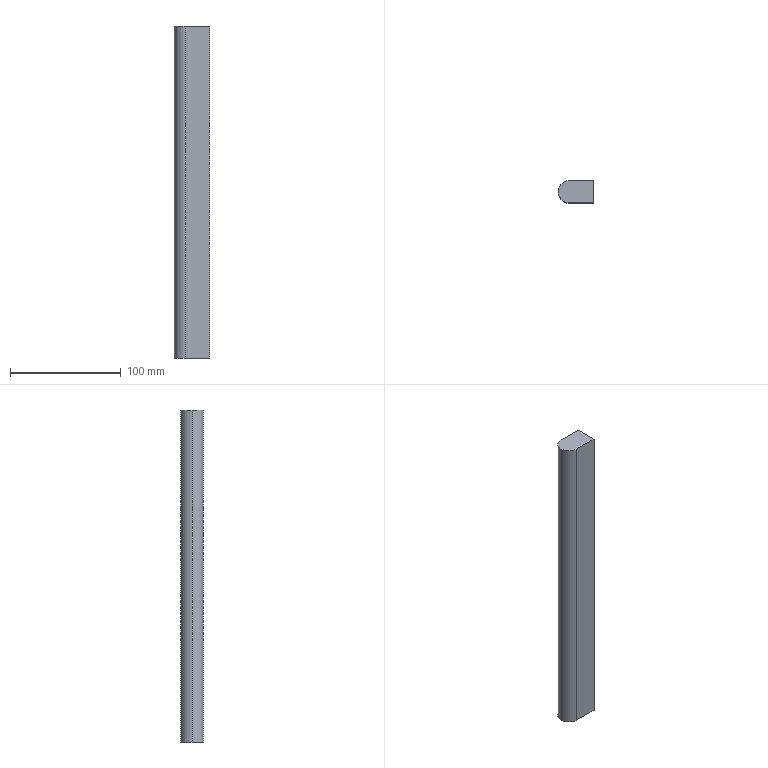Part | STEP file | Part 9 | 1 solid | 7 faces | box 32 x 20 x 300 mm | volume 179124 mm3 | plane 5 | cylinder 2 | commonest cylinder face diameters 20 x2
STEP:
#1=CARTESIAN_POINT('',(-10.,0.,300.));
#2=VERTEX_POINT('',#1);
#3=CARTESIAN_POINT('',(0.,-10.,300.));
#4=VERTEX_POINT('',#3);
#5=CARTESIAN_POINT('',(0.,0.,300.));
#6=DIRECTION('',(0.,0.,1.));
#7=DIRECTION('',(1.,0.,0.));
#8=AXIS2_PLACEMENT_3D('',#5,#6,#7);
#9=CIRCLE('',#8,10.);
#10=EDGE_CURVE('',#2,#4,#9,.T.);
#11=ORIENTED_EDGE('',*,*,#10,.F.);
#12=CARTESIAN_POINT('',(-10.,0.,0.));
#13=VERTEX_POINT('',#12);
#14=CARTESIAN_POINT('',(-10.,0.,300.));
#15=DIRECTION('',(0.,0.,-1.));
#16=VECTOR('',#15,1000.);
#17=LINE('',#14,#16);
#18=EDGE_CURVE('',#2,#13,#17,.T.);
#19=ORIENTED_EDGE('',*,*,#18,.T.);
#20=CARTESIAN_POINT('',(0.,-10.,0.));
#21=VERTEX_POINT('',#20);
#22=CARTESIAN_POINT('',(0.,0.,0.));
#23=DIRECTION('',(0.,0.,1.));
#24=DIRECTION('',(1.,0.,0.));
#25=AXIS2_PLACEMENT_3D('',#22,#23,#24);
#26=CIRCLE('',#25,10.);
#27=EDGE_CURVE('',#13,#21,#26,.T.);
#28=ORIENTED_EDGE('',*,*,#27,.T.);
#29=CARTESIAN_POINT('',(0.,-10.,300.));
#30=DIRECTION('',(0.,0.,-1.));
#31=VECTOR('',#30,1000.);
#32=LINE('',#29,#31);
#33=EDGE_CURVE('',#4,#21,#32,.T.);
#34=ORIENTED_EDGE('',*,*,#33,.F.);
#35=EDGE_LOOP('',(#11,#19,#28,#34));
#36=FACE_OUTER_BOUND('',#35,.T.);
#37=CARTESIAN_POINT('',(0.,0.,300.));
#38=DIRECTION('',(0.,0.,-1.));
#39=DIRECTION('',(-1.,0.,0.));
#40=AXIS2_PLACEMENT_3D('',#37,#38,#39);
#41=CYLINDRICAL_SURFACE('',#40,10.);
#42=ADVANCED_FACE('',(#36),#41,.T.);
#43=ORIENTED_EDGE('',*,*,#18,.F.);
#44=CARTESIAN_POINT('',(0.,10.,300.));
#45=VERTEX_POINT('',#44);
#46=CARTESIAN_POINT('',(0.,0.,300.));
#47=DIRECTION('',(0.,0.,1.));
#48=DIRECTION('',(1.,0.,0.));
#49=AXIS2_PLACEMENT_3D('',#46,#47,#48);
#50=CIRCLE('',#49,10.);
#51=EDGE_CURVE('',#45,#2,#50,.T.);
#52=ORIENTED_EDGE('',*,*,#51,.F.);
#53=CARTESIAN_POINT('',(0.,10.,0.));
#54=VERTEX_POINT('',#53);
#55=CARTESIAN_POINT('',(0.,10.,300.));
#56=DIRECTION('',(0.,0.,1.));
#57=VECTOR('',#56,1000.);
#58=LINE('',#55,#57);
#59=EDGE_CURVE('',#54,#45,#58,.T.);
#60=ORIENTED_EDGE('',*,*,#59,.F.);
#61=CARTESIAN_POINT('',(0.,0.,0.));
#62=DIRECTION('',(0.,0.,1.));
#63=DIRECTION('',(1.,0.,0.));
#64=AXIS2_PLACEMENT_3D('',#61,#62,#63);
#65=CIRCLE('',#64,10.);
#66=EDGE_CURVE('',#54,#13,#65,.T.);
#67=ORIENTED_EDGE('',*,*,#66,.T.);
#68=EDGE_LOOP('',(#43,#52,#60,#67));
#69=FACE_OUTER_BOUND('',#68,.T.);
#70=CARTESIAN_POINT('',(0.,0.,300.));
#71=DIRECTION('',(0.,0.,-1.));
#72=DIRECTION('',(-1.,0.,0.));
#73=AXIS2_PLACEMENT_3D('',#70,#71,#72);
#74=CYLINDRICAL_SURFACE('',#73,10.);
#75=ADVANCED_FACE('',(#69),#74,.T.);
#76=ORIENTED_EDGE('',*,*,#51,.T.);
#77=ORIENTED_EDGE('',*,*,#10,.T.);
#78=CARTESIAN_POINT('',(22.,-10.,300.));
#79=VERTEX_POINT('',#78);
#80=CARTESIAN_POINT('',(22.,-10.,300.));
#81=DIRECTION('',(-1.,0.,0.));
#82=VECTOR('',#81,1000.);
#83=LINE('',#80,#82);
#84=EDGE_CURVE('',#79,#4,#83,.T.);
#85=ORIENTED_EDGE('',*,*,#84,.F.);
#86=CARTESIAN_POINT('',(22.,10.,300.));
#87=VERTEX_POINT('',#86);
#88=CARTESIAN_POINT('',(22.,10.,300.));
#89=DIRECTION('',(0.,-1.,0.));
#90=VECTOR('',#89,1000.);
#91=LINE('',#88,#90);
#92=EDGE_CURVE('',#87,#79,#91,.T.);
#93=ORIENTED_EDGE('',*,*,#92,.F.);
#94=CARTESIAN_POINT('',(22.,10.,300.));
#95=DIRECTION('',(-1.,0.,0.));
#96=VECTOR('',#95,1000.);
#97=LINE('',#94,#96);
#98=EDGE_CURVE('',#87,#45,#97,.T.);
#99=ORIENTED_EDGE('',*,*,#98,.T.);
#100=EDGE_LOOP('',(#76,#77,#85,#93,#99));
#101=FACE_OUTER_BOUND('',#100,.T.);
#102=CARTESIAN_POINT('',(0.,0.,300.));
#103=DIRECTION('',(0.,0.,1.));
#104=DIRECTION('',(1.,0.,0.));
#105=AXIS2_PLACEMENT_3D('',#102,#103,#104);
#106=PLANE('',#105);
#107=ADVANCED_FACE('',(#101),#106,.T.);
#108=ORIENTED_EDGE('',*,*,#66,.F.);
#109=CARTESIAN_POINT('',(22.,10.,0.));
#110=VERTEX_POINT('',#109);
#111=CARTESIAN_POINT('',(22.,10.,0.));
#112=DIRECTION('',(-1.,0.,0.));
#113=VECTOR('',#112,1000.);
#114=LINE('',#111,#113);
#115=EDGE_CURVE('',#110,#54,#114,.T.);
#116=ORIENTED_EDGE('',*,*,#115,.F.);
#117=CARTESIAN_POINT('',(22.,-10.,0.));
#118=VERTEX_POINT('',#117);
#119=CARTESIAN_POINT('',(22.,10.,0.));
#120=DIRECTION('',(0.,1.,0.));
#121=VECTOR('',#120,1000.);
#122=LINE('',#119,#121);
#123=EDGE_CURVE('',#118,#110,#122,.T.);
#124=ORIENTED_EDGE('',*,*,#123,.F.);
#125=CARTESIAN_POINT('',(22.,-10.,0.));
#126=DIRECTION('',(-1.,0.,0.));
#127=VECTOR('',#126,1000.);
#128=LINE('',#125,#127);
#129=EDGE_CURVE('',#118,#21,#128,.T.);
#130=ORIENTED_EDGE('',*,*,#129,.T.);
#131=ORIENTED_EDGE('',*,*,#27,.F.);
#132=EDGE_LOOP('',(#108,#116,#124,#130,#131));
#133=FACE_OUTER_BOUND('',#132,.T.);
#134=CARTESIAN_POINT('',(0.,0.,0.));
#135=DIRECTION('',(0.,0.,1.));
#136=DIRECTION('',(1.,0.,0.));
#137=AXIS2_PLACEMENT_3D('',#134,#135,#136);
#138=PLANE('',#137);
#139=ADVANCED_FACE('',(#133),#138,.F.);
#140=ORIENTED_EDGE('',*,*,#33,.T.);
#141=ORIENTED_EDGE('',*,*,#129,.F.);
#142=CARTESIAN_POINT('',(22.,-10.,300.));
#143=DIRECTION('',(0.,0.,-1.));
#144=VECTOR('',#143,1000.);
#145=LINE('',#142,#144);
#146=EDGE_CURVE('',#79,#118,#145,.T.);
#147=ORIENTED_EDGE('',*,*,#146,.F.);
#148=ORIENTED_EDGE('',*,*,#84,.T.);
#149=EDGE_LOOP('',(#140,#141,#147,#148));
#150=FACE_OUTER_BOUND('',#149,.T.);
#151=CARTESIAN_POINT('',(22.,-10.,300.));
#152=DIRECTION('',(0.,1.,0.));
#153=DIRECTION('',(0.,0.,1.));
#154=AXIS2_PLACEMENT_3D('',#151,#152,#153);
#155=PLANE('',#154);
#156=ADVANCED_FACE('',(#150),#155,.F.);
#157=ORIENTED_EDGE('',*,*,#59,.T.);
#158=ORIENTED_EDGE('',*,*,#98,.F.);
#159=CARTESIAN_POINT('',(22.,10.,300.));
#160=DIRECTION('',(0.,0.,1.));
#161=VECTOR('',#160,1000.);
#162=LINE('',#159,#161);
#163=EDGE_CURVE('',#110,#87,#162,.T.);
#164=ORIENTED_EDGE('',*,*,#163,.F.);
#165=ORIENTED_EDGE('',*,*,#115,.T.);
#166=EDGE_LOOP('',(#157,#158,#164,#165));
#167=FACE_OUTER_BOUND('',#166,.T.);
#168=CARTESIAN_POINT('',(22.,10.,300.));
#169=DIRECTION('',(0.,-1.,0.));
#170=DIRECTION('',(0.,0.,-1.));
#171=AXIS2_PLACEMENT_3D('',#168,#169,#170);
#172=PLANE('',#171);
#173=ADVANCED_FACE('',(#167),#172,.F.);
#174=ORIENTED_EDGE('',*,*,#92,.T.);
#175=ORIENTED_EDGE('',*,*,#146,.T.);
#176=ORIENTED_EDGE('',*,*,#123,.T.);
#177=ORIENTED_EDGE('',*,*,#163,.T.);
#178=EDGE_LOOP('',(#174,#175,#176,#177));
#179=FACE_OUTER_BOUND('',#178,.T.);
#180=CARTESIAN_POINT('',(22.,0.,0.));
#181=DIRECTION('',(1.,0.,0.));
#182=DIRECTION('',(0.,0.,-1.));
#183=AXIS2_PLACEMENT_3D('',#180,#181,#182);
#184=PLANE('',#183);
#185=ADVANCED_FACE('',(#179),#184,.T.);
#186=CLOSED_SHELL('',(#42,#75,#107,#139,#156,#173,#185));
#187=MANIFOLD_SOLID_BREP('',#186);
#188=CARTESIAN_POINT('',(0.,0.,0.));
#189=DIRECTION('',(0.,0.,1.));
#190=DIRECTION('',(1.,0.,0.));
#191=AXIS2_PLACEMENT_3D('',#188,#189,#190);
#192=(LENGTH_UNIT()NAMED_UNIT(*)SI_UNIT(.MILLI.,.METRE.));
#193=UNCERTAINTY_MEASURE_WITH_UNIT(LENGTH_MEASURE(0.00001),#192,'','');
#194=(NAMED_UNIT(*)PLANE_ANGLE_UNIT()SI_UNIT($,.RADIAN.));
#195=(NAMED_UNIT(*)SI_UNIT($,.STERADIAN.)SOLID_ANGLE_UNIT());
#196=(GEOMETRIC_REPRESENTATION_CONTEXT(3)GLOBAL_UNCERTAINTY_ASSIGNED_CONTEXT((#193))GLOBAL_UNIT_ASSIGNED_CONTEXT((#192,#194,#195))REPRESENTATION_CONTEXT('',''));
#197=ADVANCED_BREP_SHAPE_REPRESENTATION('',(#187,#191),#196);